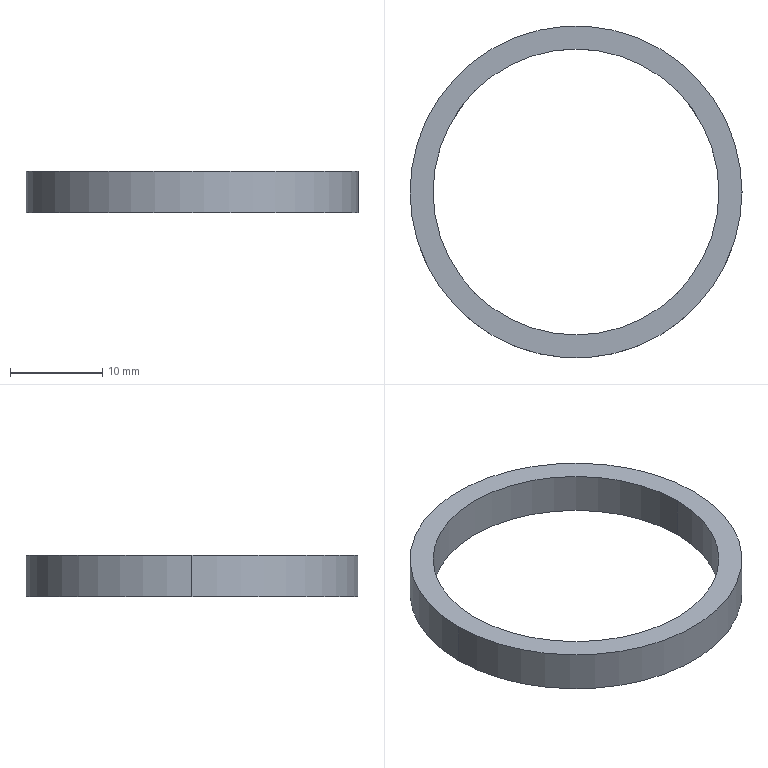Part | SolidWorks | features Extrusion 1 | 1 solid | 6 faces | box 36 x 36 x 4.5 mm | volume 1184 mm3 | cylinder 4 | plane 2 | commonest cylinder face diameters 31 x2 36 x2
STEP:
#1=CARTESIAN_POINT('',(-15.5,0.,4.5));
#2=VERTEX_POINT('',#1);
#3=CARTESIAN_POINT('',(15.5,0.,4.5));
#4=VERTEX_POINT('',#3);
#5=CARTESIAN_POINT('',(0.,0.,4.5));
#6=DIRECTION('',(0.,0.,1.));
#7=DIRECTION('',(1.,0.,0.));
#8=AXIS2_PLACEMENT_3D('',#5,#6,#7);
#9=CIRCLE('',#8,15.5);
#10=EDGE_CURVE('',#2,#4,#9,.T.);
#11=ORIENTED_EDGE('',*,*,#10,.T.);
#12=CARTESIAN_POINT('',(15.5,0.,0.));
#13=VERTEX_POINT('',#12);
#14=CARTESIAN_POINT('',(15.5,0.,4.5));
#15=DIRECTION('',(0.,0.,-1.));
#16=VECTOR('',#15,1000.);
#17=LINE('',#14,#16);
#18=EDGE_CURVE('',#4,#13,#17,.T.);
#19=ORIENTED_EDGE('',*,*,#18,.T.);
#20=CARTESIAN_POINT('',(-15.5,0.,0.));
#21=VERTEX_POINT('',#20);
#22=CARTESIAN_POINT('',(0.,0.,0.));
#23=DIRECTION('',(0.,0.,1.));
#24=DIRECTION('',(1.,0.,0.));
#25=AXIS2_PLACEMENT_3D('',#22,#23,#24);
#26=CIRCLE('',#25,15.5);
#27=EDGE_CURVE('',#21,#13,#26,.T.);
#28=ORIENTED_EDGE('',*,*,#27,.F.);
#29=CARTESIAN_POINT('',(-15.5,0.,4.5));
#30=DIRECTION('',(0.,0.,-1.));
#31=VECTOR('',#30,1000.);
#32=LINE('',#29,#31);
#33=EDGE_CURVE('',#2,#21,#32,.T.);
#34=ORIENTED_EDGE('',*,*,#33,.F.);
#35=EDGE_LOOP('',(#11,#19,#28,#34));
#36=FACE_OUTER_BOUND('',#35,.T.);
#37=CARTESIAN_POINT('',(0.,0.,4.5));
#38=DIRECTION('',(0.,0.,-1.));
#39=DIRECTION('',(-1.,0.,0.));
#40=AXIS2_PLACEMENT_3D('',#37,#38,#39);
#41=CYLINDRICAL_SURFACE('',#40,15.5);
#42=ADVANCED_FACE('',(#36),#41,.F.);
#43=CARTESIAN_POINT('',(18.,0.,4.5));
#44=VERTEX_POINT('',#43);
#45=CARTESIAN_POINT('',(-18.,0.,4.5));
#46=VERTEX_POINT('',#45);
#47=CARTESIAN_POINT('',(0.,0.,4.5));
#48=DIRECTION('',(0.,0.,1.));
#49=DIRECTION('',(1.,0.,0.));
#50=AXIS2_PLACEMENT_3D('',#47,#48,#49);
#51=CIRCLE('',#50,18.);
#52=EDGE_CURVE('',#44,#46,#51,.T.);
#53=ORIENTED_EDGE('',*,*,#52,.F.);
#54=CARTESIAN_POINT('',(18.,0.,0.));
#55=VERTEX_POINT('',#54);
#56=CARTESIAN_POINT('',(18.,0.,4.5));
#57=DIRECTION('',(0.,0.,-1.));
#58=VECTOR('',#57,1000.);
#59=LINE('',#56,#58);
#60=EDGE_CURVE('',#44,#55,#59,.T.);
#61=ORIENTED_EDGE('',*,*,#60,.T.);
#62=CARTESIAN_POINT('',(-18.,0.,0.));
#63=VERTEX_POINT('',#62);
#64=CARTESIAN_POINT('',(0.,0.,0.));
#65=DIRECTION('',(0.,0.,1.));
#66=DIRECTION('',(1.,0.,0.));
#67=AXIS2_PLACEMENT_3D('',#64,#65,#66);
#68=CIRCLE('',#67,18.);
#69=EDGE_CURVE('',#55,#63,#68,.T.);
#70=ORIENTED_EDGE('',*,*,#69,.T.);
#71=CARTESIAN_POINT('',(-18.,0.,4.5));
#72=DIRECTION('',(0.,0.,-1.));
#73=VECTOR('',#72,1000.);
#74=LINE('',#71,#73);
#75=EDGE_CURVE('',#46,#63,#74,.T.);
#76=ORIENTED_EDGE('',*,*,#75,.F.);
#77=EDGE_LOOP('',(#53,#61,#70,#76));
#78=FACE_OUTER_BOUND('',#77,.T.);
#79=CARTESIAN_POINT('',(0.,0.,4.5));
#80=DIRECTION('',(0.,0.,-1.));
#81=DIRECTION('',(-1.,0.,0.));
#82=AXIS2_PLACEMENT_3D('',#79,#80,#81);
#83=CYLINDRICAL_SURFACE('',#82,18.);
#84=ADVANCED_FACE('',(#78),#83,.T.);
#85=CARTESIAN_POINT('',(0.,0.,4.5));
#86=DIRECTION('',(0.,0.,1.));
#87=DIRECTION('',(1.,0.,0.));
#88=AXIS2_PLACEMENT_3D('',#85,#86,#87);
#89=CIRCLE('',#88,18.);
#90=EDGE_CURVE('',#46,#44,#89,.T.);
#91=ORIENTED_EDGE('',*,*,#90,.T.);
#92=ORIENTED_EDGE('',*,*,#52,.T.);
#93=EDGE_LOOP('',(#91,#92));
#94=FACE_OUTER_BOUND('',#93,.T.);
#95=ORIENTED_EDGE('',*,*,#10,.F.);
#96=CARTESIAN_POINT('',(0.,0.,4.5));
#97=DIRECTION('',(0.,0.,1.));
#98=DIRECTION('',(1.,0.,0.));
#99=AXIS2_PLACEMENT_3D('',#96,#97,#98);
#100=CIRCLE('',#99,15.5);
#101=EDGE_CURVE('',#4,#2,#100,.T.);
#102=ORIENTED_EDGE('',*,*,#101,.F.);
#103=EDGE_LOOP('',(#95,#102));
#104=FACE_BOUND('',#103,.T.);
#105=CARTESIAN_POINT('',(0.,0.,4.5));
#106=DIRECTION('',(0.,0.,1.));
#107=DIRECTION('',(1.,0.,0.));
#108=AXIS2_PLACEMENT_3D('',#105,#106,#107);
#109=PLANE('',#108);
#110=ADVANCED_FACE('',(#94,#104),#109,.T.);
#111=CARTESIAN_POINT('',(0.,0.,0.));
#112=DIRECTION('',(0.,0.,1.));
#113=DIRECTION('',(1.,0.,0.));
#114=AXIS2_PLACEMENT_3D('',#111,#112,#113);
#115=CIRCLE('',#114,18.);
#116=EDGE_CURVE('',#63,#55,#115,.T.);
#117=ORIENTED_EDGE('',*,*,#116,.F.);
#118=ORIENTED_EDGE('',*,*,#69,.F.);
#119=EDGE_LOOP('',(#117,#118));
#120=FACE_OUTER_BOUND('',#119,.T.);
#121=ORIENTED_EDGE('',*,*,#27,.T.);
#122=CARTESIAN_POINT('',(0.,0.,0.));
#123=DIRECTION('',(0.,0.,1.));
#124=DIRECTION('',(1.,0.,0.));
#125=AXIS2_PLACEMENT_3D('',#122,#123,#124);
#126=CIRCLE('',#125,15.5);
#127=EDGE_CURVE('',#13,#21,#126,.T.);
#128=ORIENTED_EDGE('',*,*,#127,.T.);
#129=EDGE_LOOP('',(#121,#128));
#130=FACE_BOUND('',#129,.T.);
#131=CARTESIAN_POINT('',(0.,0.,0.));
#132=DIRECTION('',(0.,0.,1.));
#133=DIRECTION('',(1.,0.,0.));
#134=AXIS2_PLACEMENT_3D('',#131,#132,#133);
#135=PLANE('',#134);
#136=ADVANCED_FACE('',(#120,#130),#135,.F.);
#137=ORIENTED_EDGE('',*,*,#60,.F.);
#138=ORIENTED_EDGE('',*,*,#90,.F.);
#139=ORIENTED_EDGE('',*,*,#75,.T.);
#140=ORIENTED_EDGE('',*,*,#116,.T.);
#141=EDGE_LOOP('',(#137,#138,#139,#140));
#142=FACE_OUTER_BOUND('',#141,.T.);
#143=CARTESIAN_POINT('',(0.,0.,4.5));
#144=DIRECTION('',(0.,0.,-1.));
#145=DIRECTION('',(-1.,0.,0.));
#146=AXIS2_PLACEMENT_3D('',#143,#144,#145);
#147=CYLINDRICAL_SURFACE('',#146,18.);
#148=ADVANCED_FACE('',(#142),#147,.T.);
#149=ORIENTED_EDGE('',*,*,#18,.F.);
#150=ORIENTED_EDGE('',*,*,#101,.T.);
#151=ORIENTED_EDGE('',*,*,#33,.T.);
#152=ORIENTED_EDGE('',*,*,#127,.F.);
#153=EDGE_LOOP('',(#149,#150,#151,#152));
#154=FACE_OUTER_BOUND('',#153,.T.);
#155=CARTESIAN_POINT('',(0.,0.,4.5));
#156=DIRECTION('',(0.,0.,-1.));
#157=DIRECTION('',(-1.,0.,0.));
#158=AXIS2_PLACEMENT_3D('',#155,#156,#157);
#159=CYLINDRICAL_SURFACE('',#158,15.5);
#160=ADVANCED_FACE('',(#154),#159,.F.);
#161=CLOSED_SHELL('',(#42,#84,#110,#136,#148,#160));
#162=MANIFOLD_SOLID_BREP('',#161);
#163=CARTESIAN_POINT('',(0.,0.,0.));
#164=DIRECTION('',(0.,0.,1.));
#165=DIRECTION('',(1.,0.,0.));
#166=AXIS2_PLACEMENT_3D('',#163,#164,#165);
#167=(LENGTH_UNIT()NAMED_UNIT(*)SI_UNIT(.MILLI.,.METRE.));
#168=UNCERTAINTY_MEASURE_WITH_UNIT(LENGTH_MEASURE(0.00001),#167,'','');
#169=(NAMED_UNIT(*)PLANE_ANGLE_UNIT()SI_UNIT($,.RADIAN.));
#170=(NAMED_UNIT(*)SI_UNIT($,.STERADIAN.)SOLID_ANGLE_UNIT());
#171=(GEOMETRIC_REPRESENTATION_CONTEXT(3)GLOBAL_UNCERTAINTY_ASSIGNED_CONTEXT((#168))GLOBAL_UNIT_ASSIGNED_CONTEXT((#167,#169,#170))REPRESENTATION_CONTEXT('',''));
#172=ADVANCED_BREP_SHAPE_REPRESENTATION('',(#162,#166),#171);